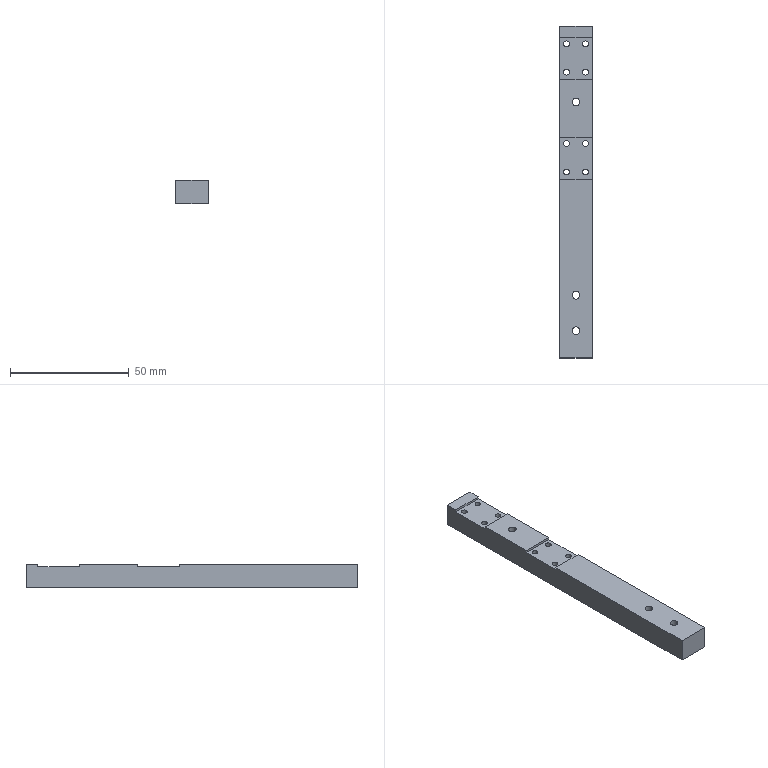Part | STEP file | PN_0003 | 1 solid | 63 faces | box 13.5 x 140 x 10 mm | volume 17518 mm3 | cylinder 40 | plane 23 | commonest cylinder face diameters 2.4 x16 4.3 x16 3.3 x6 8.05 x2